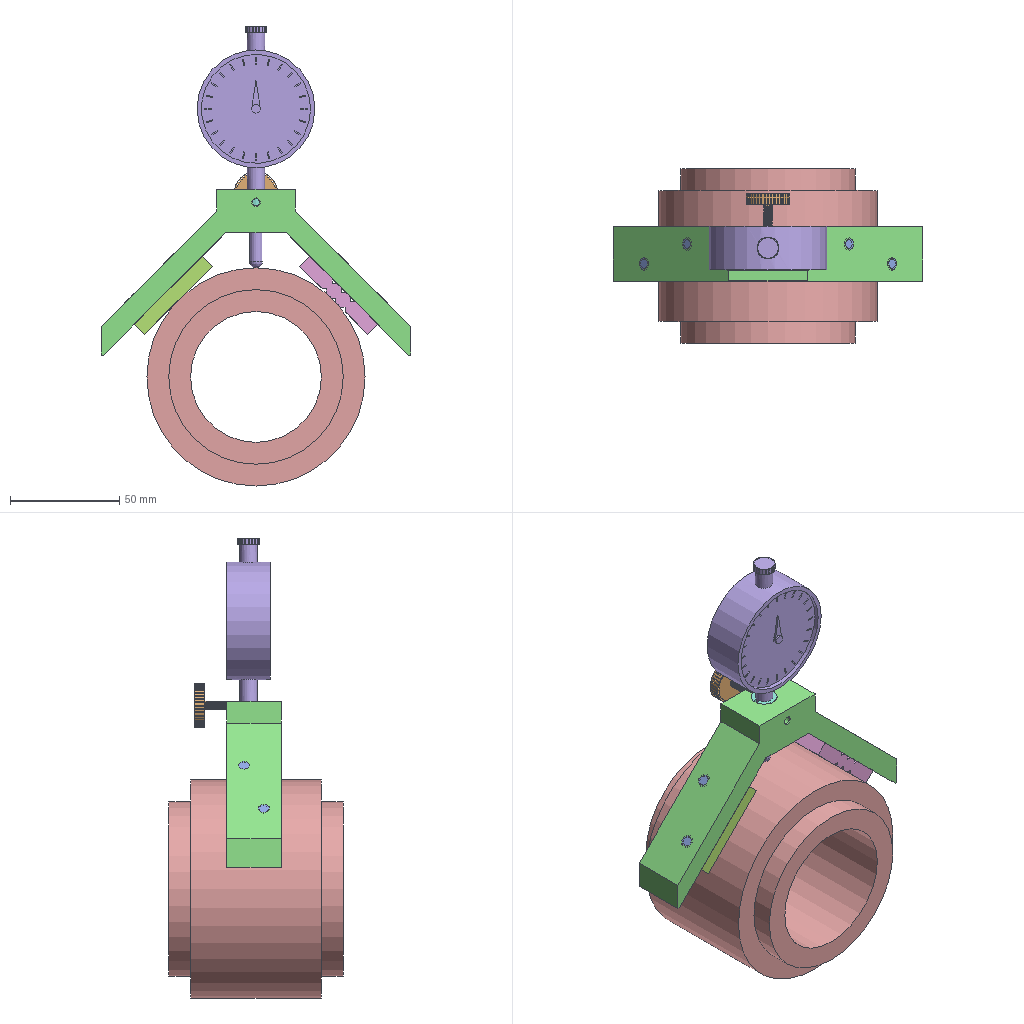Assembly | NX | 8 different items | 11 placed | box 142 x 80 x 211 mm
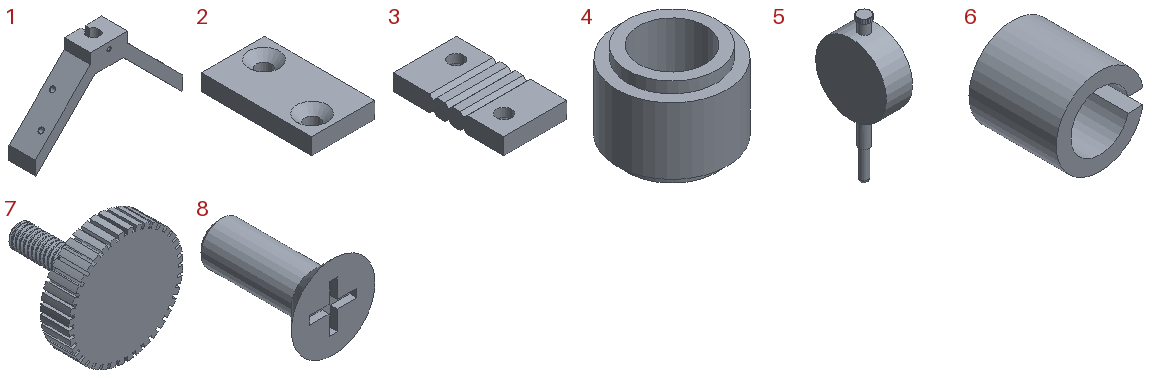Parts list (item | quantity | size | volume | features):
1 | x1 | 142 x 25 x 76 mm | 53307 mm3 | features DATUM_CSYS 8, SKETCH 7, SIMPLE HOLE 5, SYMBOLIC_THREAD 5, HOLE PACKAGE 4, EXTRUDE 3, EXTRACT_FACE 2, CBORE_HOLE 1, Instance Feature 1, Mirror Feature 1
2 | x1 | 25 x 44 x 6.5 mm | 6556 mm3 | features DATUM_CSYS 5, SKETCH 4, DATUM_PLANE 2, SWP104 2, EXTRUDE 1
3 | x1 | 25 x 44 x 6.5 mm | 6256 mm3 | features DATUM_CSYS 6, SKETCH 5, EXTRUDE 3, DATUM_PLANE 2, EXTRACT_STRING 2, SWP104 2, BREP 1, Instance Feature 1, Mirror Feature 1, TRIM BODY 1, UNITE 1
4 | x1 | 100 x 100 x 80 mm | 345575 mm3 | features DATUM_CSYS 3, EXTRUDE 2, SKETCH 2, HOLE PACKAGE 1, SIMPLE HOLE 1
5 | x1 | 20 x 54 x 110.9 mm | 44306 mm3 | features EXTRUDE 30, EXTRACT_STRING 24, Instance Feature 23, DATUM_CSYS 7, SKETCH 6, CYLINDER 3, DATUM_PLANE 1, OFFSET_CURVE 1, Pattern Feature 1, SPHERE 1
6 | x1 | 11.916 x 12 x 12 mm | 705.642 mm3 | features DATUM_CSYS 3, EXTRUDE 2, SKETCH 2
7 | x1 | 19.994 x 19 x 19.994 mm | 1639 mm3 | features DATUM_CSYS 3, SKETCH 2, CHAMFER 1, DATUM_PLANE 1, EXTRUDE 1, SWP104 1, THREADS 1
8 | x4 | 12 x 16.5 x 12 mm | 562.519 mm3 | features DATUM_CSYS 3, SKETCH 2, CHAMFER 1, EXTRUDE 1, SWP104 1
Mates (type | each side: item.copy, entity, surface, feature):
Fix | 1.1 component
Touch | 6.1 face cylinder Extrude(2) | 1.1 face cylinder Ø8 Counterbored Hole(5)
Concentric | 6.1 edge | 1.1 edge
Distance | 7.1 face plane Revolve(1) | 1.1 face plane Extrude(2)
Touch | 2.1 face cone Revolve(7) | 1.1 face cylinder Mirror Feature(8)
Touch | 8.1 face cylinder Revolve(1) | 2.1 face cone Revolve(6)
Touch | 8.1 face cylinder Revolve(1) | 2.1 face cone Revolve(7)
Concentric | 8.1 edge | 2.1 edge | 2 times
Touch | 3.1 face cylinder Revolve(6) | 1.1 face cylinder M5 x 0.8 Threaded Hole(7)
Touch | 3.1 face plane Trim Body(10) | 1.1 face plane Extrude(4)
Touch | 8.1 face cylinder Revolve(1) | 3.1 face cylinder Revolve(7)
Touch | 8.1 face cylinder Revolve(1) | 3.1 face cylinder Revolve(6)
Concentric | 8.1 edge | 3.1 edge | 2 times
Perpendicular | 4.1 face cylinder Extrude(4) | 6.1 face cylinder Extrude(2)
Touch | 4.1 face cylinder Extrude(4) | 2.1 face plane Extrude(2)
Touch | 4.1 face cylinder Extrude(4) | 3.1 face plane Body(8)
Touch | 5.1 face sphere Sphere(1) | 4.1 face cylinder Extrude(4)
Touch | 5.1 face cylinder Cylinder(3) | 6.1 face cylinder Extrude(2)